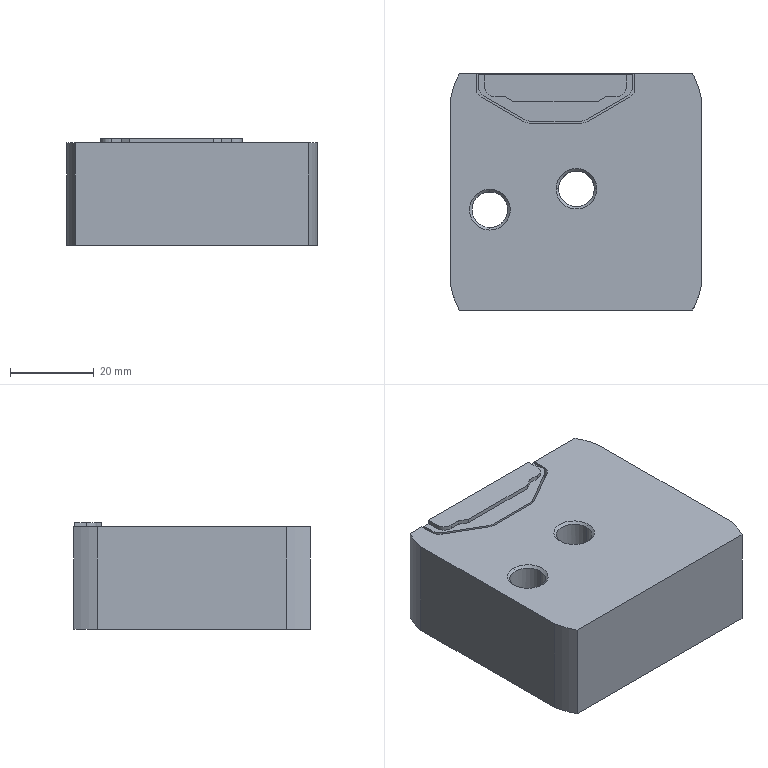Part | STEP file | DGC-25-G right fixed end | 1 solid | 146 faces | box 59.8 x 56.5 x 25.5 mm | volume 73184 mm3 | cylinder 63 | plane 47 | cone 24 | spline 12 | commonest cylinder face diameters 3 x10 5 x10 17.4 x10 8.566 x8 12.8 x8 4.134 x6